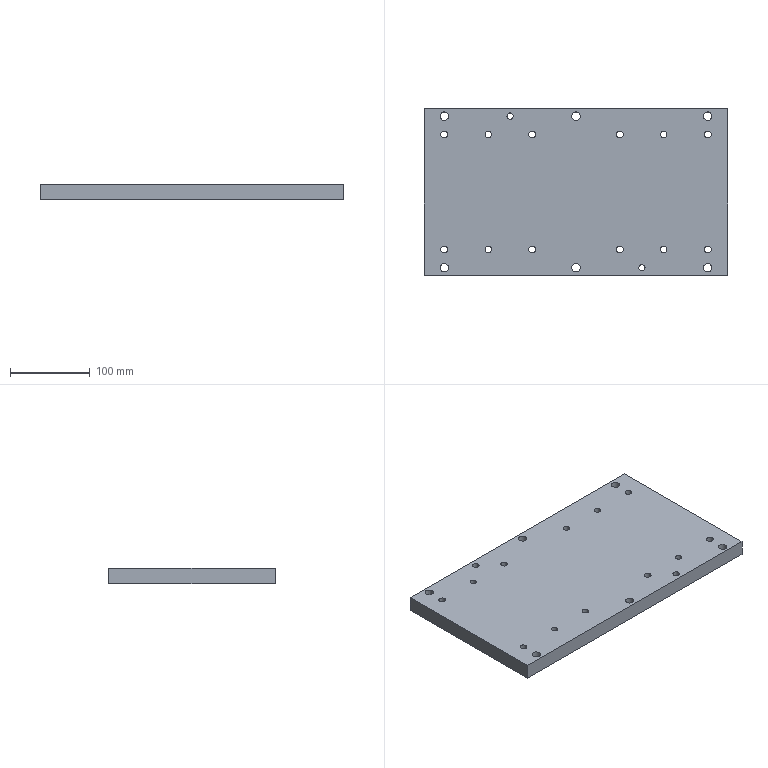Part | STEP file | Tube feed_id1770_x_t | 1 solid | 42 faces | box 380 x 208.2 x 19.5 mm | volume 1510900 mm3 | cylinder 28 | plane 14 | commonest cylinder face diameters 8.5 x8 14 x8 8 x6 10.5 x6